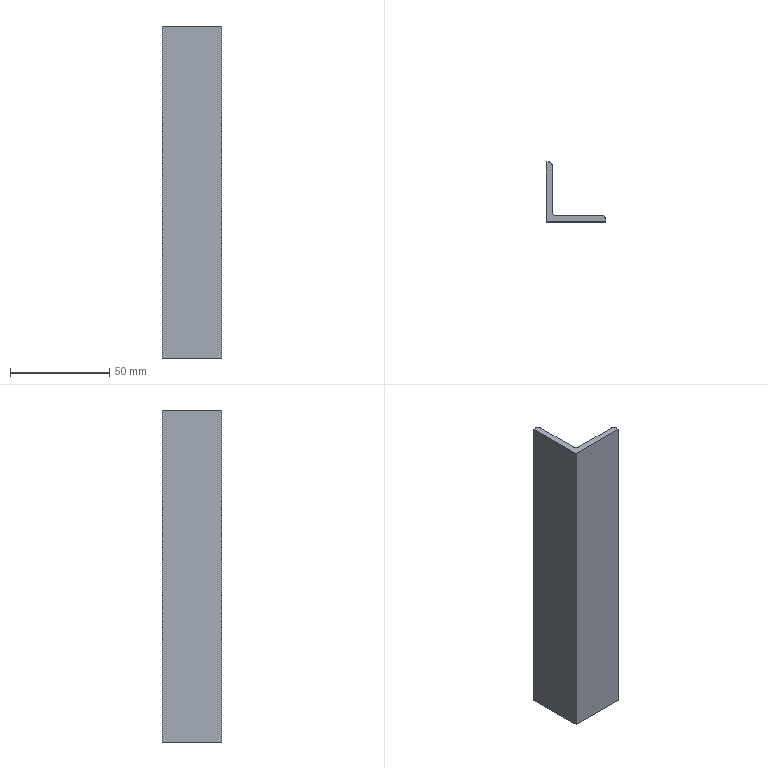Part | SolidWorks | features Extrusion 1 | 1 solid | 11 faces | box 30 x 30 x 167 mm | volume 28414 mm3 | plane 8 | cylinder 3 | commonest cylinder face diameters 4 x3
STEP:
#1=CARTESIAN_POINT('',(0.,30.,0.));
#2=VERTEX_POINT('',#1);
#3=CARTESIAN_POINT('',(0.,0.,0.));
#4=VERTEX_POINT('',#3);
#5=CARTESIAN_POINT('',(0.,0.,0.));
#6=DIRECTION('',(0.,-1.,0.));
#7=VECTOR('',#6,1000.);
#8=LINE('',#5,#7);
#9=EDGE_CURVE('',#2,#4,#8,.T.);
#10=ORIENTED_EDGE('',*,*,#9,.T.);
#11=CARTESIAN_POINT('',(0.,0.,167.));
#12=VERTEX_POINT('',#11);
#13=CARTESIAN_POINT('',(0.,0.,167.));
#14=DIRECTION('',(0.,0.,-1.));
#15=VECTOR('',#14,1000.);
#16=LINE('',#13,#15);
#17=EDGE_CURVE('',#12,#4,#16,.T.);
#18=ORIENTED_EDGE('',*,*,#17,.F.);
#19=CARTESIAN_POINT('',(0.,30.,167.));
#20=VERTEX_POINT('',#19);
#21=CARTESIAN_POINT('',(0.,0.,167.));
#22=DIRECTION('',(0.,-1.,0.));
#23=VECTOR('',#22,1000.);
#24=LINE('',#21,#23);
#25=EDGE_CURVE('',#20,#12,#24,.T.);
#26=ORIENTED_EDGE('',*,*,#25,.F.);
#27=CARTESIAN_POINT('',(0.,30.,167.));
#28=DIRECTION('',(0.,0.,-1.));
#29=VECTOR('',#28,1000.);
#30=LINE('',#27,#29);
#31=EDGE_CURVE('',#20,#2,#30,.T.);
#32=ORIENTED_EDGE('',*,*,#31,.T.);
#33=EDGE_LOOP('',(#10,#18,#26,#32));
#34=FACE_OUTER_BOUND('',#33,.T.);
#35=CARTESIAN_POINT('',(0.,0.,167.));
#36=DIRECTION('',(1.,0.,0.));
#37=DIRECTION('',(0.,0.,-1.));
#38=AXIS2_PLACEMENT_3D('',#35,#36,#37);
#39=PLANE('',#38);
#40=ADVANCED_FACE('',(#34),#39,.F.);
#41=CARTESIAN_POINT('',(30.,0.,0.));
#42=VERTEX_POINT('',#41);
#43=CARTESIAN_POINT('',(0.,0.,0.));
#44=DIRECTION('',(1.,0.,0.));
#45=VECTOR('',#44,1000.);
#46=LINE('',#43,#45);
#47=EDGE_CURVE('',#4,#42,#46,.T.);
#48=ORIENTED_EDGE('',*,*,#47,.T.);
#49=CARTESIAN_POINT('',(30.,0.,167.));
#50=VERTEX_POINT('',#49);
#51=CARTESIAN_POINT('',(30.,0.,167.));
#52=DIRECTION('',(0.,0.,-1.));
#53=VECTOR('',#52,1000.);
#54=LINE('',#51,#53);
#55=EDGE_CURVE('',#50,#42,#54,.T.);
#56=ORIENTED_EDGE('',*,*,#55,.F.);
#57=CARTESIAN_POINT('',(0.,0.,167.));
#58=DIRECTION('',(1.,0.,0.));
#59=VECTOR('',#58,1000.);
#60=LINE('',#57,#59);
#61=EDGE_CURVE('',#12,#50,#60,.T.);
#62=ORIENTED_EDGE('',*,*,#61,.F.);
#63=ORIENTED_EDGE('',*,*,#17,.T.);
#64=EDGE_LOOP('',(#48,#56,#62,#63));
#65=FACE_OUTER_BOUND('',#64,.T.);
#66=CARTESIAN_POINT('',(0.,0.,167.));
#67=DIRECTION('',(0.,1.,0.));
#68=DIRECTION('',(0.,0.,1.));
#69=AXIS2_PLACEMENT_3D('',#66,#67,#68);
#70=PLANE('',#69);
#71=ADVANCED_FACE('',(#65),#70,.F.);
#72=CARTESIAN_POINT('',(30.,1.,0.));
#73=VERTEX_POINT('',#72);
#74=CARTESIAN_POINT('',(30.,1.,0.));
#75=DIRECTION('',(0.,1.,0.));
#76=VECTOR('',#75,1000.);
#77=LINE('',#74,#76);
#78=EDGE_CURVE('',#42,#73,#77,.T.);
#79=ORIENTED_EDGE('',*,*,#78,.T.);
#80=CARTESIAN_POINT('',(30.,1.,167.));
#81=VERTEX_POINT('',#80);
#82=CARTESIAN_POINT('',(30.,1.,167.));
#83=DIRECTION('',(0.,0.,-1.));
#84=VECTOR('',#83,1000.);
#85=LINE('',#82,#84);
#86=EDGE_CURVE('',#81,#73,#85,.T.);
#87=ORIENTED_EDGE('',*,*,#86,.F.);
#88=CARTESIAN_POINT('',(30.,1.,167.));
#89=DIRECTION('',(0.,1.,0.));
#90=VECTOR('',#89,1000.);
#91=LINE('',#88,#90);
#92=EDGE_CURVE('',#50,#81,#91,.T.);
#93=ORIENTED_EDGE('',*,*,#92,.F.);
#94=ORIENTED_EDGE('',*,*,#55,.T.);
#95=EDGE_LOOP('',(#79,#87,#93,#94));
#96=FACE_OUTER_BOUND('',#95,.T.);
#97=CARTESIAN_POINT('',(30.,1.,167.));
#98=DIRECTION('',(-1.,0.,0.));
#99=DIRECTION('',(0.,0.,1.));
#100=AXIS2_PLACEMENT_3D('',#97,#98,#99);
#101=PLANE('',#100);
#102=ADVANCED_FACE('',(#96),#101,.F.);
#103=CARTESIAN_POINT('',(28.,3.,0.));
#104=VERTEX_POINT('',#103);
#105=CARTESIAN_POINT('',(28.,1.,0.));
#106=DIRECTION('',(0.,0.,1.));
#107=DIRECTION('',(1.,0.,0.));
#108=AXIS2_PLACEMENT_3D('',#105,#106,#107);
#109=CIRCLE('',#108,2.);
#110=EDGE_CURVE('',#73,#104,#109,.T.);
#111=ORIENTED_EDGE('',*,*,#110,.T.);
#112=CARTESIAN_POINT('',(28.,3.,167.));
#113=VERTEX_POINT('',#112);
#114=CARTESIAN_POINT('',(28.,3.,167.));
#115=DIRECTION('',(0.,0.,-1.));
#116=VECTOR('',#115,1000.);
#117=LINE('',#114,#116);
#118=EDGE_CURVE('',#113,#104,#117,.T.);
#119=ORIENTED_EDGE('',*,*,#118,.F.);
#120=CARTESIAN_POINT('',(28.,1.,167.));
#121=DIRECTION('',(0.,0.,1.));
#122=DIRECTION('',(1.,0.,0.));
#123=AXIS2_PLACEMENT_3D('',#120,#121,#122);
#124=CIRCLE('',#123,2.);
#125=EDGE_CURVE('',#81,#113,#124,.T.);
#126=ORIENTED_EDGE('',*,*,#125,.F.);
#127=ORIENTED_EDGE('',*,*,#86,.T.);
#128=EDGE_LOOP('',(#111,#119,#126,#127));
#129=FACE_OUTER_BOUND('',#128,.T.);
#130=CARTESIAN_POINT('',(28.,1.,167.));
#131=DIRECTION('',(0.,0.,-1.));
#132=DIRECTION('',(-1.,0.,0.));
#133=AXIS2_PLACEMENT_3D('',#130,#131,#132);
#134=CYLINDRICAL_SURFACE('',#133,2.);
#135=ADVANCED_FACE('',(#129),#134,.T.);
#136=CARTESIAN_POINT('',(5.,3.,0.));
#137=VERTEX_POINT('',#136);
#138=CARTESIAN_POINT('',(5.,3.,0.));
#139=DIRECTION('',(-1.,0.,0.));
#140=VECTOR('',#139,1000.);
#141=LINE('',#138,#140);
#142=EDGE_CURVE('',#104,#137,#141,.T.);
#143=ORIENTED_EDGE('',*,*,#142,.T.);
#144=CARTESIAN_POINT('',(5.,3.,167.));
#145=VERTEX_POINT('',#144);
#146=CARTESIAN_POINT('',(5.,3.,167.));
#147=DIRECTION('',(0.,0.,-1.));
#148=VECTOR('',#147,1000.);
#149=LINE('',#146,#148);
#150=EDGE_CURVE('',#145,#137,#149,.T.);
#151=ORIENTED_EDGE('',*,*,#150,.F.);
#152=CARTESIAN_POINT('',(5.,3.,167.));
#153=DIRECTION('',(-1.,0.,0.));
#154=VECTOR('',#153,1000.);
#155=LINE('',#152,#154);
#156=EDGE_CURVE('',#113,#145,#155,.T.);
#157=ORIENTED_EDGE('',*,*,#156,.F.);
#158=ORIENTED_EDGE('',*,*,#118,.T.);
#159=EDGE_LOOP('',(#143,#151,#157,#158));
#160=FACE_OUTER_BOUND('',#159,.T.);
#161=CARTESIAN_POINT('',(5.,3.,167.));
#162=DIRECTION('',(0.,-1.,0.));
#163=DIRECTION('',(0.,0.,-1.));
#164=AXIS2_PLACEMENT_3D('',#161,#162,#163);
#165=PLANE('',#164);
#166=ADVANCED_FACE('',(#160),#165,.F.);
#167=CARTESIAN_POINT('',(3.,5.,0.));
#168=VERTEX_POINT('',#167);
#169=CARTESIAN_POINT('',(5.,5.,0.));
#170=DIRECTION('',(0.,0.,-1.));
#171=DIRECTION('',(-1.,0.,0.));
#172=AXIS2_PLACEMENT_3D('',#169,#170,#171);
#173=CIRCLE('',#172,2.);
#174=EDGE_CURVE('',#137,#168,#173,.T.);
#175=ORIENTED_EDGE('',*,*,#174,.T.);
#176=CARTESIAN_POINT('',(3.,5.,167.));
#177=VERTEX_POINT('',#176);
#178=CARTESIAN_POINT('',(3.,5.,167.));
#179=DIRECTION('',(0.,0.,-1.));
#180=VECTOR('',#179,1000.);
#181=LINE('',#178,#180);
#182=EDGE_CURVE('',#177,#168,#181,.T.);
#183=ORIENTED_EDGE('',*,*,#182,.F.);
#184=CARTESIAN_POINT('',(5.,5.,167.));
#185=DIRECTION('',(0.,0.,-1.));
#186=DIRECTION('',(-1.,0.,0.));
#187=AXIS2_PLACEMENT_3D('',#184,#185,#186);
#188=CIRCLE('',#187,2.);
#189=EDGE_CURVE('',#145,#177,#188,.T.);
#190=ORIENTED_EDGE('',*,*,#189,.F.);
#191=ORIENTED_EDGE('',*,*,#150,.T.);
#192=EDGE_LOOP('',(#175,#183,#190,#191));
#193=FACE_OUTER_BOUND('',#192,.T.);
#194=CARTESIAN_POINT('',(5.,5.,167.));
#195=DIRECTION('',(0.,0.,-1.));
#196=DIRECTION('',(-1.,0.,0.));
#197=AXIS2_PLACEMENT_3D('',#194,#195,#196);
#198=CYLINDRICAL_SURFACE('',#197,2.);
#199=ADVANCED_FACE('',(#193),#198,.F.);
#200=CARTESIAN_POINT('',(3.,28.,0.));
#201=VERTEX_POINT('',#200);
#202=CARTESIAN_POINT('',(3.,5.,0.));
#203=DIRECTION('',(0.,1.,0.));
#204=VECTOR('',#203,1000.);
#205=LINE('',#202,#204);
#206=EDGE_CURVE('',#168,#201,#205,.T.);
#207=ORIENTED_EDGE('',*,*,#206,.T.);
#208=CARTESIAN_POINT('',(3.,28.,167.));
#209=VERTEX_POINT('',#208);
#210=CARTESIAN_POINT('',(3.,28.,167.));
#211=DIRECTION('',(0.,0.,-1.));
#212=VECTOR('',#211,1000.);
#213=LINE('',#210,#212);
#214=EDGE_CURVE('',#209,#201,#213,.T.);
#215=ORIENTED_EDGE('',*,*,#214,.F.);
#216=CARTESIAN_POINT('',(3.,5.,167.));
#217=DIRECTION('',(0.,1.,0.));
#218=VECTOR('',#217,1000.);
#219=LINE('',#216,#218);
#220=EDGE_CURVE('',#177,#209,#219,.T.);
#221=ORIENTED_EDGE('',*,*,#220,.F.);
#222=ORIENTED_EDGE('',*,*,#182,.T.);
#223=EDGE_LOOP('',(#207,#215,#221,#222));
#224=FACE_OUTER_BOUND('',#223,.T.);
#225=CARTESIAN_POINT('',(3.,5.,167.));
#226=DIRECTION('',(-1.,0.,0.));
#227=DIRECTION('',(0.,0.,1.));
#228=AXIS2_PLACEMENT_3D('',#225,#226,#227);
#229=PLANE('',#228);
#230=ADVANCED_FACE('',(#224),#229,.F.);
#231=CARTESIAN_POINT('',(1.,30.,0.));
#232=VERTEX_POINT('',#231);
#233=CARTESIAN_POINT('',(1.,28.,0.));
#234=DIRECTION('',(0.,0.,1.));
#235=DIRECTION('',(-1.,0.,0.));
#236=AXIS2_PLACEMENT_3D('',#233,#234,#235);
#237=CIRCLE('',#236,2.);
#238=EDGE_CURVE('',#201,#232,#237,.T.);
#239=ORIENTED_EDGE('',*,*,#238,.T.);
#240=CARTESIAN_POINT('',(1.,30.,167.));
#241=VERTEX_POINT('',#240);
#242=CARTESIAN_POINT('',(1.,30.,167.));
#243=DIRECTION('',(0.,0.,-1.));
#244=VECTOR('',#243,1000.);
#245=LINE('',#242,#244);
#246=EDGE_CURVE('',#241,#232,#245,.T.);
#247=ORIENTED_EDGE('',*,*,#246,.F.);
#248=CARTESIAN_POINT('',(1.,28.,167.));
#249=DIRECTION('',(0.,0.,1.));
#250=DIRECTION('',(-1.,0.,0.));
#251=AXIS2_PLACEMENT_3D('',#248,#249,#250);
#252=CIRCLE('',#251,2.);
#253=EDGE_CURVE('',#209,#241,#252,.T.);
#254=ORIENTED_EDGE('',*,*,#253,.F.);
#255=ORIENTED_EDGE('',*,*,#214,.T.);
#256=EDGE_LOOP('',(#239,#247,#254,#255));
#257=FACE_OUTER_BOUND('',#256,.T.);
#258=CARTESIAN_POINT('',(1.,28.,167.));
#259=DIRECTION('',(0.,0.,-1.));
#260=DIRECTION('',(-1.,0.,0.));
#261=AXIS2_PLACEMENT_3D('',#258,#259,#260);
#262=CYLINDRICAL_SURFACE('',#261,2.);
#263=ADVANCED_FACE('',(#257),#262,.T.);
#264=CARTESIAN_POINT('',(0.,30.,0.));
#265=DIRECTION('',(-1.,0.,0.));
#266=VECTOR('',#265,1000.);
#267=LINE('',#264,#266);
#268=EDGE_CURVE('',#232,#2,#267,.T.);
#269=ORIENTED_EDGE('',*,*,#268,.T.);
#270=ORIENTED_EDGE('',*,*,#31,.F.);
#271=CARTESIAN_POINT('',(0.,30.,167.));
#272=DIRECTION('',(-1.,0.,0.));
#273=VECTOR('',#272,1000.);
#274=LINE('',#271,#273);
#275=EDGE_CURVE('',#241,#20,#274,.T.);
#276=ORIENTED_EDGE('',*,*,#275,.F.);
#277=ORIENTED_EDGE('',*,*,#246,.T.);
#278=EDGE_LOOP('',(#269,#270,#276,#277));
#279=FACE_OUTER_BOUND('',#278,.T.);
#280=CARTESIAN_POINT('',(0.,30.,167.));
#281=DIRECTION('',(0.,-1.,0.));
#282=DIRECTION('',(0.,0.,-1.));
#283=AXIS2_PLACEMENT_3D('',#280,#281,#282);
#284=PLANE('',#283);
#285=ADVANCED_FACE('',(#279),#284,.F.);
#286=ORIENTED_EDGE('',*,*,#25,.T.);
#287=ORIENTED_EDGE('',*,*,#61,.T.);
#288=ORIENTED_EDGE('',*,*,#92,.T.);
#289=ORIENTED_EDGE('',*,*,#125,.T.);
#290=ORIENTED_EDGE('',*,*,#156,.T.);
#291=ORIENTED_EDGE('',*,*,#189,.T.);
#292=ORIENTED_EDGE('',*,*,#220,.T.);
#293=ORIENTED_EDGE('',*,*,#253,.T.);
#294=ORIENTED_EDGE('',*,*,#275,.T.);
#295=EDGE_LOOP('',(#286,#287,#288,#289,#290,#291,#292,#293,#294));
#296=FACE_OUTER_BOUND('',#295,.T.);
#297=CARTESIAN_POINT('',(1.,28.,167.));
#298=DIRECTION('',(0.,0.,-1.));
#299=DIRECTION('',(-1.,0.,0.));
#300=AXIS2_PLACEMENT_3D('',#297,#298,#299);
#301=PLANE('',#300);
#302=ADVANCED_FACE('',(#296),#301,.F.);
#303=ORIENTED_EDGE('',*,*,#9,.F.);
#304=ORIENTED_EDGE('',*,*,#268,.F.);
#305=ORIENTED_EDGE('',*,*,#238,.F.);
#306=ORIENTED_EDGE('',*,*,#206,.F.);
#307=ORIENTED_EDGE('',*,*,#174,.F.);
#308=ORIENTED_EDGE('',*,*,#142,.F.);
#309=ORIENTED_EDGE('',*,*,#110,.F.);
#310=ORIENTED_EDGE('',*,*,#78,.F.);
#311=ORIENTED_EDGE('',*,*,#47,.F.);
#312=EDGE_LOOP('',(#303,#304,#305,#306,#307,#308,#309,#310,#311));
#313=FACE_OUTER_BOUND('',#312,.T.);
#314=CARTESIAN_POINT('',(1.,28.,0.));
#315=DIRECTION('',(0.,0.,-1.));
#316=DIRECTION('',(-1.,0.,0.));
#317=AXIS2_PLACEMENT_3D('',#314,#315,#316);
#318=PLANE('',#317);
#319=ADVANCED_FACE('',(#313),#318,.T.);
#320=CLOSED_SHELL('',(#40,#71,#102,#135,#166,#199,#230,#263,#285,#302,#319));
#321=MANIFOLD_SOLID_BREP('',#320);
#322=CARTESIAN_POINT('',(0.,0.,0.));
#323=DIRECTION('',(0.,0.,1.));
#324=DIRECTION('',(1.,0.,0.));
#325=AXIS2_PLACEMENT_3D('',#322,#323,#324);
#326=(LENGTH_UNIT()NAMED_UNIT(*)SI_UNIT(.MILLI.,.METRE.));
#327=UNCERTAINTY_MEASURE_WITH_UNIT(LENGTH_MEASURE(0.00001),#326,'','');
#328=(NAMED_UNIT(*)PLANE_ANGLE_UNIT()SI_UNIT($,.RADIAN.));
#329=(NAMED_UNIT(*)SI_UNIT($,.STERADIAN.)SOLID_ANGLE_UNIT());
#330=(GEOMETRIC_REPRESENTATION_CONTEXT(3)GLOBAL_UNCERTAINTY_ASSIGNED_CONTEXT((#327))GLOBAL_UNIT_ASSIGNED_CONTEXT((#326,#328,#329))REPRESENTATION_CONTEXT('',''));
#331=ADVANCED_BREP_SHAPE_REPRESENTATION('',(#321,#325),#330);